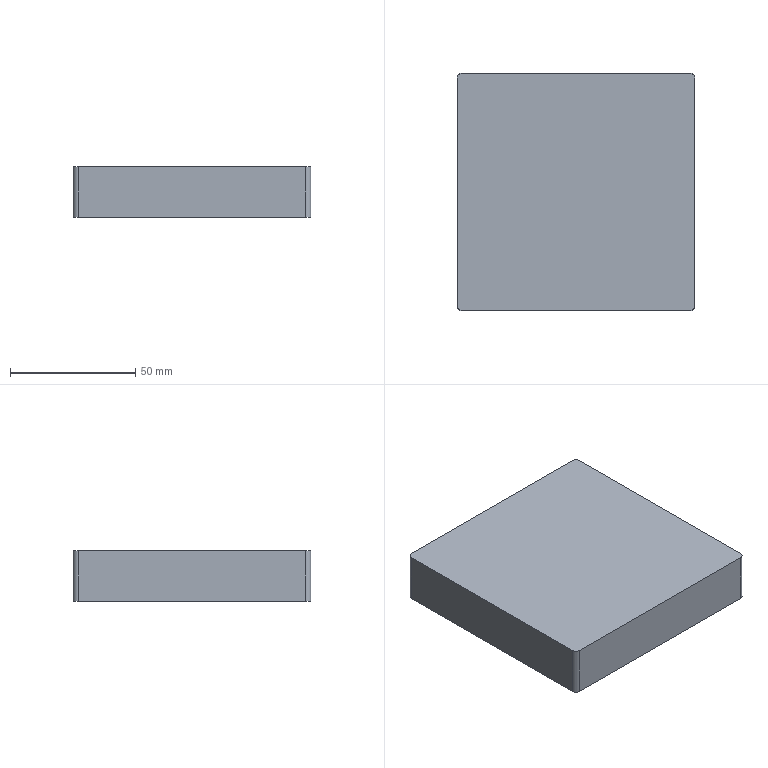Part | NX | features solid 2 | 1 solid | 13 faces | box 95 x 95 x 20 mm | volume 178892 mm3 | plane 8 | cylinder 5 | commonest cylinder face diameters 4 x4 14 x1
STEP:
#1=CARTESIAN_POINT('',(245.5,-137.5,-413.));
#2=VERTEX_POINT('',#1);
#3=CARTESIAN_POINT('',(154.5,-137.5,-413.));
#4=VERTEX_POINT('',#3);
#5=CARTESIAN_POINT('',(247.5,-137.5,-413.));
#6=DIRECTION('',(-1.,0.,0.));
#7=VECTOR('',#6,1000.);
#8=LINE('',#5,#7);
#9=EDGE_CURVE('',#2,#4,#8,.T.);
#10=ORIENTED_EDGE('',*,*,#9,.F.);
#11=CARTESIAN_POINT('',(245.5,-137.5,-393.));
#12=VERTEX_POINT('',#11);
#13=CARTESIAN_POINT('',(245.5,-137.5,-413.));
#14=DIRECTION('',(0.,0.,1.));
#15=VECTOR('',#14,1000.);
#16=LINE('',#13,#15);
#17=EDGE_CURVE('',#2,#12,#16,.T.);
#18=ORIENTED_EDGE('',*,*,#17,.T.);
#19=CARTESIAN_POINT('',(154.5,-137.5,-393.));
#20=VERTEX_POINT('',#19);
#21=CARTESIAN_POINT('',(247.5,-137.5,-393.));
#22=DIRECTION('',(-1.,0.,0.));
#23=VECTOR('',#22,1000.);
#24=LINE('',#21,#23);
#25=EDGE_CURVE('',#12,#20,#24,.T.);
#26=ORIENTED_EDGE('',*,*,#25,.T.);
#27=CARTESIAN_POINT('',(154.5,-137.5,-413.));
#28=DIRECTION('',(0.,0.,1.));
#29=VECTOR('',#28,1000.);
#30=LINE('',#27,#29);
#31=EDGE_CURVE('',#20,#4,#30,.F.);
#32=ORIENTED_EDGE('',*,*,#31,.T.);
#33=EDGE_LOOP('',(#10,#18,#26,#32));
#34=FACE_BOUND('',#33,.T.);
#35=CARTESIAN_POINT('',(247.5,-137.5,-413.));
#36=DIRECTION('',(0.,1.,0.));
#37=DIRECTION('',(0.,0.,1.));
#38=AXIS2_PLACEMENT_3D('',#35,#36,#37);
#39=PLANE('',#38);
#40=ADVANCED_FACE('',(#34),#39,.F.);
#41=CARTESIAN_POINT('',(152.5,-135.5,-393.));
#42=VERTEX_POINT('',#41);
#43=CARTESIAN_POINT('',(152.5,-44.5,-393.));
#44=VERTEX_POINT('',#43);
#45=CARTESIAN_POINT('',(152.5,-137.5,-393.));
#46=DIRECTION('',(0.,1.,0.));
#47=VECTOR('',#46,1000.);
#48=LINE('',#45,#47);
#49=EDGE_CURVE('',#42,#44,#48,.T.);
#50=ORIENTED_EDGE('',*,*,#49,.T.);
#51=CARTESIAN_POINT('',(152.5,-44.5,-413.));
#52=VERTEX_POINT('',#51);
#53=CARTESIAN_POINT('',(152.5,-44.5,-413.));
#54=DIRECTION('',(0.,0.,1.));
#55=VECTOR('',#54,1000.);
#56=LINE('',#53,#55);
#57=EDGE_CURVE('',#44,#52,#56,.F.);
#58=ORIENTED_EDGE('',*,*,#57,.T.);
#59=CARTESIAN_POINT('',(152.5,-135.5,-413.));
#60=VERTEX_POINT('',#59);
#61=CARTESIAN_POINT('',(152.5,-137.5,-413.));
#62=DIRECTION('',(0.,1.,0.));
#63=VECTOR('',#62,1000.);
#64=LINE('',#61,#63);
#65=EDGE_CURVE('',#60,#52,#64,.T.);
#66=ORIENTED_EDGE('',*,*,#65,.F.);
#67=CARTESIAN_POINT('',(152.5,-135.5,-413.));
#68=DIRECTION('',(0.,0.,1.));
#69=VECTOR('',#68,1000.);
#70=LINE('',#67,#69);
#71=EDGE_CURVE('',#60,#42,#70,.T.);
#72=ORIENTED_EDGE('',*,*,#71,.T.);
#73=EDGE_LOOP('',(#50,#58,#66,#72));
#74=FACE_BOUND('',#73,.T.);
#75=CARTESIAN_POINT('',(152.5,-137.5,-413.));
#76=DIRECTION('',(1.,0.,0.));
#77=DIRECTION('',(0.,1.,0.));
#78=AXIS2_PLACEMENT_3D('',#75,#76,#77);
#79=PLANE('',#78);
#80=ADVANCED_FACE('',(#74),#79,.F.);
#81=CARTESIAN_POINT('',(154.5,-42.5,-393.));
#82=VERTEX_POINT('',#81);
#83=CARTESIAN_POINT('',(245.5,-42.5,-393.));
#84=VERTEX_POINT('',#83);
#85=CARTESIAN_POINT('',(152.5,-42.5,-393.));
#86=DIRECTION('',(1.,0.,0.));
#87=VECTOR('',#86,1000.);
#88=LINE('',#85,#87);
#89=EDGE_CURVE('',#82,#84,#88,.T.);
#90=ORIENTED_EDGE('',*,*,#89,.T.);
#91=CARTESIAN_POINT('',(245.5,-42.5,-413.));
#92=VERTEX_POINT('',#91);
#93=CARTESIAN_POINT('',(245.5,-42.5,-413.));
#94=DIRECTION('',(0.,0.,1.));
#95=VECTOR('',#94,1000.);
#96=LINE('',#93,#95);
#97=EDGE_CURVE('',#84,#92,#96,.F.);
#98=ORIENTED_EDGE('',*,*,#97,.T.);
#99=CARTESIAN_POINT('',(154.5,-42.5,-413.));
#100=VERTEX_POINT('',#99);
#101=CARTESIAN_POINT('',(152.5,-42.5,-413.));
#102=DIRECTION('',(1.,0.,0.));
#103=VECTOR('',#102,1000.);
#104=LINE('',#101,#103);
#105=EDGE_CURVE('',#100,#92,#104,.T.);
#106=ORIENTED_EDGE('',*,*,#105,.F.);
#107=CARTESIAN_POINT('',(154.5,-42.5,-413.));
#108=DIRECTION('',(0.,0.,1.));
#109=VECTOR('',#108,1000.);
#110=LINE('',#107,#109);
#111=EDGE_CURVE('',#100,#82,#110,.T.);
#112=ORIENTED_EDGE('',*,*,#111,.T.);
#113=EDGE_LOOP('',(#90,#98,#106,#112));
#114=FACE_BOUND('',#113,.T.);
#115=CARTESIAN_POINT('',(152.5,-42.5,-413.));
#116=DIRECTION('',(0.,-1.,0.));
#117=DIRECTION('',(0.,0.,-1.));
#118=AXIS2_PLACEMENT_3D('',#115,#116,#117);
#119=PLANE('',#118);
#120=ADVANCED_FACE('',(#114),#119,.F.);
#121=CARTESIAN_POINT('',(247.5,-44.5,-413.));
#122=VERTEX_POINT('',#121);
#123=CARTESIAN_POINT('',(247.5,-135.5,-413.));
#124=VERTEX_POINT('',#123);
#125=CARTESIAN_POINT('',(247.5,-42.5,-413.));
#126=DIRECTION('',(0.,-1.,0.));
#127=VECTOR('',#126,1000.);
#128=LINE('',#125,#127);
#129=EDGE_CURVE('',#122,#124,#128,.T.);
#130=ORIENTED_EDGE('',*,*,#129,.F.);
#131=CARTESIAN_POINT('',(247.5,-44.5,-393.));
#132=VERTEX_POINT('',#131);
#133=CARTESIAN_POINT('',(247.5,-44.5,-413.));
#134=DIRECTION('',(0.,0.,1.));
#135=VECTOR('',#134,1000.);
#136=LINE('',#133,#135);
#137=EDGE_CURVE('',#122,#132,#136,.T.);
#138=ORIENTED_EDGE('',*,*,#137,.T.);
#139=CARTESIAN_POINT('',(247.5,-135.5,-393.));
#140=VERTEX_POINT('',#139);
#141=CARTESIAN_POINT('',(247.5,-42.5,-393.));
#142=DIRECTION('',(0.,-1.,0.));
#143=VECTOR('',#142,1000.);
#144=LINE('',#141,#143);
#145=EDGE_CURVE('',#132,#140,#144,.T.);
#146=ORIENTED_EDGE('',*,*,#145,.T.);
#147=CARTESIAN_POINT('',(247.5,-135.5,-413.));
#148=DIRECTION('',(0.,0.,1.));
#149=VECTOR('',#148,1000.);
#150=LINE('',#147,#149);
#151=EDGE_CURVE('',#140,#124,#150,.F.);
#152=ORIENTED_EDGE('',*,*,#151,.T.);
#153=EDGE_LOOP('',(#130,#138,#146,#152));
#154=FACE_BOUND('',#153,.T.);
#155=CARTESIAN_POINT('',(247.5,-42.5,-413.));
#156=DIRECTION('',(-1.,0.,0.));
#157=DIRECTION('',(0.,-1.,0.));
#158=AXIS2_PLACEMENT_3D('',#155,#156,#157);
#159=PLANE('',#158);
#160=ADVANCED_FACE('',(#154),#159,.F.);
#161=ORIENTED_EDGE('',*,*,#105,.T.);
#162=CARTESIAN_POINT('',(245.5,-44.5,-413.));
#163=DIRECTION('',(0.,0.,-1.));
#164=DIRECTION('',(0.,1.,0.));
#165=AXIS2_PLACEMENT_3D('',#162,#163,#164);
#166=CIRCLE('',#165,2.);
#167=EDGE_CURVE('',#92,#122,#166,.T.);
#168=ORIENTED_EDGE('',*,*,#167,.T.);
#169=ORIENTED_EDGE('',*,*,#129,.T.);
#170=CARTESIAN_POINT('',(245.5,-135.5,-413.));
#171=DIRECTION('',(0.,0.,-1.));
#172=DIRECTION('',(0.,1.,0.));
#173=AXIS2_PLACEMENT_3D('',#170,#171,#172);
#174=CIRCLE('',#173,2.);
#175=EDGE_CURVE('',#124,#2,#174,.T.);
#176=ORIENTED_EDGE('',*,*,#175,.T.);
#177=ORIENTED_EDGE('',*,*,#9,.T.);
#178=CARTESIAN_POINT('',(154.5,-135.5,-413.));
#179=DIRECTION('',(0.,0.,-1.));
#180=DIRECTION('',(0.,1.,0.));
#181=AXIS2_PLACEMENT_3D('',#178,#179,#180);
#182=CIRCLE('',#181,2.);
#183=EDGE_CURVE('',#4,#60,#182,.T.);
#184=ORIENTED_EDGE('',*,*,#183,.T.);
#185=ORIENTED_EDGE('',*,*,#65,.T.);
#186=CARTESIAN_POINT('',(154.5,-44.5,-413.));
#187=DIRECTION('',(0.,0.,-1.));
#188=DIRECTION('',(0.,1.,0.));
#189=AXIS2_PLACEMENT_3D('',#186,#187,#188);
#190=CIRCLE('',#189,2.);
#191=EDGE_CURVE('',#52,#100,#190,.T.);
#192=ORIENTED_EDGE('',*,*,#191,.T.);
#193=EDGE_LOOP('',(#161,#168,#169,#176,#177,#184,#185,#192));
#194=FACE_BOUND('',#193,.T.);
#195=CARTESIAN_POINT('',(152.5,-137.5,-413.));
#196=DIRECTION('',(0.,0.,-1.));
#197=DIRECTION('',(0.,1.,0.));
#198=AXIS2_PLACEMENT_3D('',#195,#196,#197);
#199=PLANE('',#198);
#200=ADVANCED_FACE('',(#194),#199,.T.);
#201=ORIENTED_EDGE('',*,*,#145,.F.);
#202=CARTESIAN_POINT('',(245.5,-44.5,-393.));
#203=DIRECTION('',(0.,0.,-1.));
#204=DIRECTION('',(0.,1.,0.));
#205=AXIS2_PLACEMENT_3D('',#202,#203,#204);
#206=CIRCLE('',#205,2.);
#207=EDGE_CURVE('',#132,#84,#206,.F.);
#208=ORIENTED_EDGE('',*,*,#207,.T.);
#209=ORIENTED_EDGE('',*,*,#89,.F.);
#210=CARTESIAN_POINT('',(154.5,-44.5,-393.));
#211=DIRECTION('',(0.,0.,-1.));
#212=DIRECTION('',(0.,1.,0.));
#213=AXIS2_PLACEMENT_3D('',#210,#211,#212);
#214=CIRCLE('',#213,2.);
#215=EDGE_CURVE('',#82,#44,#214,.F.);
#216=ORIENTED_EDGE('',*,*,#215,.T.);
#217=ORIENTED_EDGE('',*,*,#49,.F.);
#218=CARTESIAN_POINT('',(154.5,-135.5,-393.));
#219=DIRECTION('',(0.,0.,-1.));
#220=DIRECTION('',(0.,1.,0.));
#221=AXIS2_PLACEMENT_3D('',#218,#219,#220);
#222=CIRCLE('',#221,2.);
#223=EDGE_CURVE('',#42,#20,#222,.F.);
#224=ORIENTED_EDGE('',*,*,#223,.T.);
#225=ORIENTED_EDGE('',*,*,#25,.F.);
#226=CARTESIAN_POINT('',(245.5,-135.5,-393.));
#227=DIRECTION('',(0.,0.,-1.));
#228=DIRECTION('',(0.,1.,0.));
#229=AXIS2_PLACEMENT_3D('',#226,#227,#228);
#230=CIRCLE('',#229,2.);
#231=EDGE_CURVE('',#12,#140,#230,.F.);
#232=ORIENTED_EDGE('',*,*,#231,.T.);
#233=EDGE_LOOP('',(#201,#208,#209,#216,#217,#224,#225,#232));
#234=FACE_BOUND('',#233,.T.);
#235=CARTESIAN_POINT('',(152.5,-137.5,-393.));
#236=DIRECTION('',(0.,0.,-1.));
#237=DIRECTION('',(0.,1.,0.));
#238=AXIS2_PLACEMENT_3D('',#235,#236,#237);
#239=PLANE('',#238);
#240=ADVANCED_FACE('',(#234),#239,.F.);
#241=ORIENTED_EDGE('',*,*,#167,.F.);
#242=ORIENTED_EDGE('',*,*,#97,.F.);
#243=ORIENTED_EDGE('',*,*,#207,.F.);
#244=ORIENTED_EDGE('',*,*,#137,.F.);
#245=EDGE_LOOP('',(#241,#242,#243,#244));
#246=FACE_BOUND('',#245,.T.);
#247=CARTESIAN_POINT('',(245.5,-44.5,-413.));
#248=DIRECTION('',(0.,0.,1.));
#249=DIRECTION('',(0.,-1.,0.));
#250=AXIS2_PLACEMENT_3D('',#247,#248,#249);
#251=CYLINDRICAL_SURFACE('',#250,2.);
#252=ADVANCED_FACE('',(#246),#251,.T.);
#253=ORIENTED_EDGE('',*,*,#191,.F.);
#254=ORIENTED_EDGE('',*,*,#57,.F.);
#255=ORIENTED_EDGE('',*,*,#215,.F.);
#256=ORIENTED_EDGE('',*,*,#111,.F.);
#257=EDGE_LOOP('',(#253,#254,#255,#256));
#258=FACE_BOUND('',#257,.T.);
#259=CARTESIAN_POINT('',(154.5,-44.5,-413.));
#260=DIRECTION('',(0.,0.,1.));
#261=DIRECTION('',(0.,-1.,0.));
#262=AXIS2_PLACEMENT_3D('',#259,#260,#261);
#263=CYLINDRICAL_SURFACE('',#262,2.);
#264=ADVANCED_FACE('',(#258),#263,.T.);
#265=ORIENTED_EDGE('',*,*,#175,.F.);
#266=ORIENTED_EDGE('',*,*,#151,.F.);
#267=ORIENTED_EDGE('',*,*,#231,.F.);
#268=ORIENTED_EDGE('',*,*,#17,.F.);
#269=EDGE_LOOP('',(#265,#266,#267,#268));
#270=FACE_BOUND('',#269,.T.);
#271=CARTESIAN_POINT('',(245.5,-135.5,-413.));
#272=DIRECTION('',(0.,0.,1.));
#273=DIRECTION('',(0.,-1.,0.));
#274=AXIS2_PLACEMENT_3D('',#271,#272,#273);
#275=CYLINDRICAL_SURFACE('',#274,2.);
#276=ADVANCED_FACE('',(#270),#275,.T.);
#277=ORIENTED_EDGE('',*,*,#183,.F.);
#278=ORIENTED_EDGE('',*,*,#31,.F.);
#279=ORIENTED_EDGE('',*,*,#223,.F.);
#280=ORIENTED_EDGE('',*,*,#71,.F.);
#281=EDGE_LOOP('',(#277,#278,#279,#280));
#282=FACE_BOUND('',#281,.T.);
#283=CARTESIAN_POINT('',(154.5,-135.5,-413.));
#284=DIRECTION('',(0.,0.,1.));
#285=DIRECTION('',(0.,-1.,0.));
#286=AXIS2_PLACEMENT_3D('',#283,#284,#285);
#287=CYLINDRICAL_SURFACE('',#286,2.);
#288=ADVANCED_FACE('',(#282),#287,.T.);
#289=CLOSED_SHELL('',(#40,#80,#120,#160,#200,#240,#252,#264,#276,#288));
#290=CARTESIAN_POINT('',(220.,-97.,-403.));
#291=VERTEX_POINT('',#290);
#292=CARTESIAN_POINT('',(220.,-90.,-403.));
#293=DIRECTION('',(1.,0.,0.));
#294=DIRECTION('',(0.,-1.,0.));
#295=AXIS2_PLACEMENT_3D('',#292,#293,#294);
#296=CIRCLE('',#295,7.);
#297=EDGE_CURVE('',#291,#291,#296,.T.);
#298=ORIENTED_EDGE('',*,*,#297,.F.);
#299=EDGE_LOOP('',(#298));
#300=FACE_BOUND('',#299,.T.);
#301=CARTESIAN_POINT('',(230.,-97.,-403.));
#302=VERTEX_POINT('',#301);
#303=CARTESIAN_POINT('',(230.,-90.,-403.));
#304=DIRECTION('',(1.,0.,0.));
#305=DIRECTION('',(0.,-1.,0.));
#306=AXIS2_PLACEMENT_3D('',#303,#304,#305);
#307=CIRCLE('',#306,7.);
#308=EDGE_CURVE('',#302,#302,#307,.T.);
#309=ORIENTED_EDGE('',*,*,#308,.T.);
#310=EDGE_LOOP('',(#309));
#311=FACE_BOUND('',#310,.T.);
#312=CARTESIAN_POINT('',(220.,-90.,-403.));
#313=DIRECTION('',(1.,0.,0.));
#314=DIRECTION('',(0.,0.,1.));
#315=AXIS2_PLACEMENT_3D('',#312,#313,#314);
#316=CYLINDRICAL_SURFACE('',#315,7.);
#317=ADVANCED_FACE('',(#300,#311),#316,.F.);
#318=ORIENTED_EDGE('',*,*,#297,.T.);
#319=EDGE_LOOP('',(#318));
#320=FACE_BOUND('',#319,.T.);
#321=CARTESIAN_POINT('',(220.,-90.,-403.));
#322=DIRECTION('',(1.,0.,0.));
#323=DIRECTION('',(0.,0.,1.));
#324=AXIS2_PLACEMENT_3D('',#321,#322,#323);
#325=PLANE('',#324);
#326=ADVANCED_FACE('',(#320),#325,.T.);
#327=ORIENTED_EDGE('',*,*,#308,.F.);
#328=EDGE_LOOP('',(#327));
#329=FACE_BOUND('',#328,.T.);
#330=CARTESIAN_POINT('',(230.,-90.,-403.));
#331=DIRECTION('',(1.,0.,0.));
#332=DIRECTION('',(0.,0.,1.));
#333=AXIS2_PLACEMENT_3D('',#330,#331,#332);
#334=PLANE('',#333);
#335=ADVANCED_FACE('',(#329),#334,.F.);
#336=CLOSED_SHELL('',(#317,#326,#335));
#337=ORIENTED_CLOSED_SHELL('',*,#336,.F.);
#338=BREP_WITH_VOIDS('',#289,(#337));
#339=(LENGTH_UNIT()NAMED_UNIT(*)SI_UNIT(.MILLI.,.METRE.));
#340=UNCERTAINTY_MEASURE_WITH_UNIT(LENGTH_MEASURE(0.00001),#339,'','');
#341=(NAMED_UNIT(*)PLANE_ANGLE_UNIT()SI_UNIT($,.RADIAN.));
#342=(NAMED_UNIT(*)SI_UNIT($,.STERADIAN.)SOLID_ANGLE_UNIT());
#343=(GEOMETRIC_REPRESENTATION_CONTEXT(3)GLOBAL_UNCERTAINTY_ASSIGNED_CONTEXT((#340))GLOBAL_UNIT_ASSIGNED_CONTEXT((#339,#341,#342))REPRESENTATION_CONTEXT('',''));
#344=ADVANCED_BREP_SHAPE_REPRESENTATION('',(#338),#343);